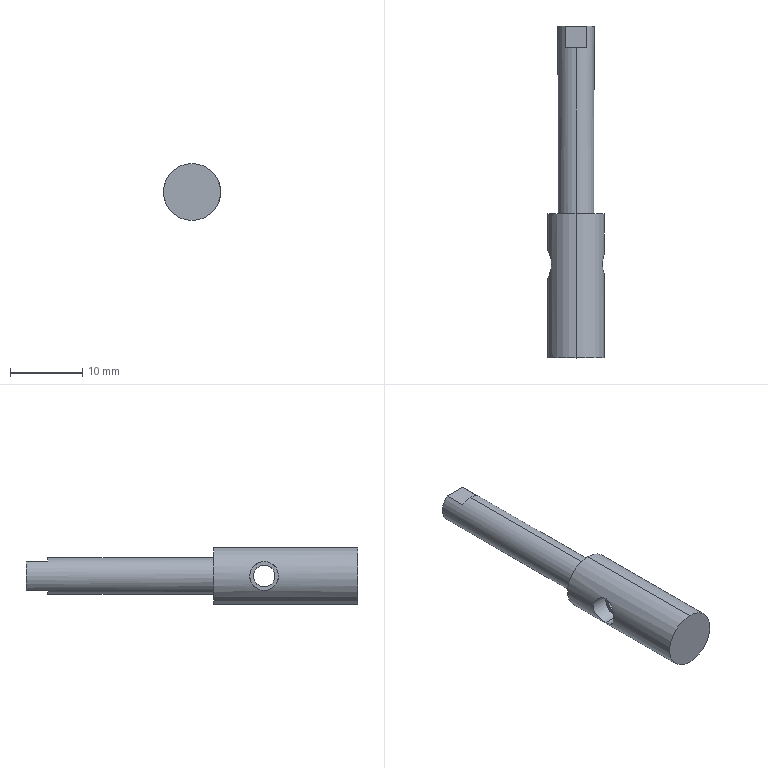Part | SolidWorks | features ICE 4, 3DProfileFeature 1, Extrusion 1, HoleWzd 1 | 1 solid | 20 faces | box 7.9 x 46 x 7.9 mm | volume 1380 mm3 | cylinder 10 | plane 8 | cone 2 | commonest cylinder face diameters 2.5 x2 3 x2 4 x2 5 x2 7.9 x2
STEP:
#1=CARTESIAN_POINT('',(0.,38.5,-1.25));
#2=VERTEX_POINT('',#1);
#3=CARTESIAN_POINT('',(0.,38.5,1.25));
#4=VERTEX_POINT('',#3);
#5=CARTESIAN_POINT('',(0.,38.5,0.));
#6=DIRECTION('',(0.,1.,0.));
#7=DIRECTION('',(0.,0.,1.));
#8=AXIS2_PLACEMENT_3D('',#5,#6,#7);
#9=CIRCLE('',#8,1.25);
#10=EDGE_CURVE('',#2,#4,#9,.T.);
#11=ORIENTED_EDGE('',*,*,#10,.F.);
#12=CARTESIAN_POINT('',(0.,46.,-1.25));
#13=VERTEX_POINT('',#12);
#14=CARTESIAN_POINT('',(0.,46.,-1.25));
#15=DIRECTION('',(0.,1.,0.));
#16=VECTOR('',#15,1000.);
#17=LINE('',#14,#16);
#18=EDGE_CURVE('',#2,#13,#17,.T.);
#19=ORIENTED_EDGE('',*,*,#18,.T.);
#20=CARTESIAN_POINT('',(0.,46.,1.25));
#21=VERTEX_POINT('',#20);
#22=CARTESIAN_POINT('',(0.,46.,0.));
#23=DIRECTION('',(0.,1.,0.));
#24=DIRECTION('',(0.,0.,1.));
#25=AXIS2_PLACEMENT_3D('',#22,#23,#24);
#26=CIRCLE('',#25,1.25);
#27=EDGE_CURVE('',#13,#21,#26,.T.);
#28=ORIENTED_EDGE('',*,*,#27,.T.);
#29=CARTESIAN_POINT('',(0.,46.,1.25));
#30=DIRECTION('',(0.,1.,0.));
#31=VECTOR('',#30,1000.);
#32=LINE('',#29,#31);
#33=EDGE_CURVE('',#4,#21,#32,.T.);
#34=ORIENTED_EDGE('',*,*,#33,.F.);
#35=EDGE_LOOP('',(#11,#19,#28,#34));
#36=FACE_OUTER_BOUND('',#35,.T.);
#37=CARTESIAN_POINT('',(0.,46.,0.));
#38=DIRECTION('',(0.,1.,0.));
#39=DIRECTION('',(0.,0.,1.));
#40=AXIS2_PLACEMENT_3D('',#37,#38,#39);
#41=CYLINDRICAL_SURFACE('',#40,1.25);
#42=ADVANCED_FACE('',(#36),#41,.F.);
#43=CARTESIAN_POINT('',(0.,37.749,0.));
#44=VERTEX_POINT('',#43);
#45=CARTESIAN_POINT('',(0.,38.5,1.25));
#46=DIRECTION('',(0.,0.515,0.8572));
#47=VECTOR('',#46,1000.);
#48=LINE('',#45,#47);
#49=EDGE_CURVE('',#44,#4,#48,.T.);
#50=ORIENTED_EDGE('',*,*,#49,.F.);
#51=CARTESIAN_POINT('',(0.,38.5,-1.25));
#52=DIRECTION('',(0.,0.515,-0.8572));
#53=VECTOR('',#52,1000.);
#54=LINE('',#51,#53);
#55=EDGE_CURVE('',#44,#2,#54,.T.);
#56=ORIENTED_EDGE('',*,*,#55,.T.);
#57=ORIENTED_EDGE('',*,*,#10,.T.);
#58=EDGE_LOOP('',(#50,#56,#57));
#59=FACE_OUTER_BOUND('',#58,.T.);
#60=CARTESIAN_POINT('',(0.,38.5,0.));
#61=DIRECTION('',(0.,1.,0.));
#62=DIRECTION('',(0.,0.,1.));
#63=AXIS2_PLACEMENT_3D('',#60,#61,#62);
#64=CONICAL_SURFACE('',#63,1.25,1.03);
#65=ADVANCED_FACE('',(#59),#64,.F.);
#66=CARTESIAN_POINT('',(-3.406,13.,2.));
#67=VERTEX_POINT('',#66);
#68=CARTESIAN_POINT('',(-3.406,13.,-2.));
#69=VERTEX_POINT('',#68);
#70=CARTESIAN_POINT('',(-3.406,13.,2.));
#71=CARTESIAN_POINT('',(-3.406,12.868,2.));
#72=CARTESIAN_POINT('',(-3.414,12.733,1.986));
#73=CARTESIAN_POINT('',(-3.444,12.473,1.934));
#74=CARTESIAN_POINT('',(-3.466,12.348,1.895));
#75=CARTESIAN_POINT('',(-3.52,12.105,1.793));
#76=CARTESIAN_POINT('',(-3.551,11.991,1.732));
#77=CARTESIAN_POINT('',(-3.618,11.777,1.588));
#78=CARTESIAN_POINT('',(-3.653,11.677,1.505));
#79=CARTESIAN_POINT('',(-3.723,11.495,1.324));
#80=CARTESIAN_POINT('',(-3.757,11.414,1.225));
#81=CARTESIAN_POINT('',(-3.82,11.269,1.01));
#82=CARTESIAN_POINT('',(-3.849,11.206,0.8939));
#83=CARTESIAN_POINT('',(-3.921,11.055,0.5341));
#84=CARTESIAN_POINT('',(-3.95,11.,0.2668));
#85=CARTESIAN_POINT('',(-3.95,11.,-0.1306));
#86=CARTESIAN_POINT('',(-3.943,11.013,-0.2652));
#87=CARTESIAN_POINT('',(-3.917,11.066,-0.5255));
#88=CARTESIAN_POINT('',(-3.898,11.104,-0.6512));
#89=CARTESIAN_POINT('',(-3.825,11.257,-1.015));
#90=CARTESIAN_POINT('',(-3.758,11.404,-1.233));
#91=CARTESIAN_POINT('',(-3.653,11.678,-1.506));
#92=CARTESIAN_POINT('',(-3.618,11.777,-1.588));
#93=CARTESIAN_POINT('',(-3.551,11.991,-1.731));
#94=CARTESIAN_POINT('',(-3.519,12.107,-1.794));
#95=CARTESIAN_POINT('',(-3.466,12.347,-1.895));
#96=CARTESIAN_POINT('',(-3.445,12.471,-1.933));
#97=CARTESIAN_POINT('',(-3.414,12.73,-1.986));
#98=CARTESIAN_POINT('',(-3.406,12.866,-2.));
#99=CARTESIAN_POINT('',(-3.406,13.,-2.));
#100=B_SPLINE_CURVE_WITH_KNOTS('',3,(#70,#71,#72,#73,#74,#75,#76,#77,#78,#79,#80,#81,#82,#83,#84,#85,#86,#87,#88,#89,#90,#91,#92,#93,#94,#95,#96,#97,#98,#99),.UNSPECIFIED.,.F.,.F.,(4,2,2,2,2,2,2,2,2,2,2,2,2,2,4),(0.006364,0.006761,0.007158,0.007555,0.007952,0.008349,0.008746,0.009541,0.009938,0.01033,0.01113,0.01153,0.01192,0.01232,0.01272),.UNSPECIFIED.);
#101=EDGE_CURVE('',#67,#69,#100,.T.);
#102=ORIENTED_EDGE('',*,*,#101,.F.);
#103=CARTESIAN_POINT('',(-1.5,13.,2.));
#104=VERTEX_POINT('',#103);
#105=CARTESIAN_POINT('',(-11.5,13.,2.));
#106=DIRECTION('',(1.,0.,0.));
#107=VECTOR('',#106,1000.);
#108=LINE('',#105,#107);
#109=EDGE_CURVE('',#67,#104,#108,.T.);
#110=ORIENTED_EDGE('',*,*,#109,.T.);
#111=CARTESIAN_POINT('',(-1.5,13.,-2.));
#112=VERTEX_POINT('',#111);
#113=CARTESIAN_POINT('',(-1.5,13.,0.));
#114=DIRECTION('',(1.,0.,0.));
#115=DIRECTION('',(0.,0.,-1.));
#116=AXIS2_PLACEMENT_3D('',#113,#114,#115);
#117=CIRCLE('',#116,2.);
#118=EDGE_CURVE('',#104,#112,#117,.T.);
#119=ORIENTED_EDGE('',*,*,#118,.T.);
#120=CARTESIAN_POINT('',(-11.5,13.,-2.));
#121=DIRECTION('',(1.,0.,0.));
#122=VECTOR('',#121,1000.);
#123=LINE('',#120,#122);
#124=EDGE_CURVE('',#69,#112,#123,.T.);
#125=ORIENTED_EDGE('',*,*,#124,.F.);
#126=EDGE_LOOP('',(#102,#110,#119,#125));
#127=FACE_OUTER_BOUND('',#126,.T.);
#128=CARTESIAN_POINT('',(-11.5,13.,0.));
#129=DIRECTION('',(1.,0.,0.));
#130=DIRECTION('',(0.,0.,-1.));
#131=AXIS2_PLACEMENT_3D('',#128,#129,#130);
#132=CYLINDRICAL_SURFACE('',#131,2.);
#133=ADVANCED_FACE('',(#127),#132,.F.);
#134=CARTESIAN_POINT('',(-1.5,13.,-1.5));
#135=VERTEX_POINT('',#134);
#136=CARTESIAN_POINT('',(-1.5,13.,1.5));
#137=VERTEX_POINT('',#136);
#138=CARTESIAN_POINT('',(-1.5,13.,0.));
#139=DIRECTION('',(-1.,0.,0.));
#140=DIRECTION('',(0.,0.,-1.));
#141=AXIS2_PLACEMENT_3D('',#138,#139,#140);
#142=CIRCLE('',#141,1.5);
#143=EDGE_CURVE('',#135,#137,#142,.T.);
#144=ORIENTED_EDGE('',*,*,#143,.T.);
#145=CARTESIAN_POINT('',(3.654,13.,1.5));
#146=VERTEX_POINT('',#145);
#147=CARTESIAN_POINT('',(-3.95,13.,1.5));
#148=DIRECTION('',(1.,0.,0.));
#149=VECTOR('',#148,1000.);
#150=LINE('',#147,#149);
#151=EDGE_CURVE('',#137,#146,#150,.T.);
#152=ORIENTED_EDGE('',*,*,#151,.T.);
#153=CARTESIAN_POINT('',(3.654,13.,-1.5));
#154=VERTEX_POINT('',#153);
#155=CARTESIAN_POINT('',(3.654,13.,-1.5));
#156=CARTESIAN_POINT('',(3.654,12.9,-1.5));
#157=CARTESIAN_POINT('',(3.658,12.802,-1.49));
#158=CARTESIAN_POINT('',(3.674,12.609,-1.451));
#159=CARTESIAN_POINT('',(3.685,12.513,-1.422));
#160=CARTESIAN_POINT('',(3.728,12.241,-1.309));
#161=CARTESIAN_POINT('',(3.767,12.076,-1.198));
#162=CARTESIAN_POINT('',(3.843,11.802,-0.9235));
#163=CARTESIAN_POINT('',(3.881,11.691,-0.7578));
#164=CARTESIAN_POINT('',(3.921,11.578,-0.4874));
#165=CARTESIAN_POINT('',(3.932,11.549,-0.3918));
#166=CARTESIAN_POINT('',(3.946,11.51,-0.1977));
#167=CARTESIAN_POINT('',(3.95,11.5,-0.09969));
#168=CARTESIAN_POINT('',(3.95,11.5,0.0982));
#169=CARTESIAN_POINT('',(3.946,11.51,0.1986));
#170=CARTESIAN_POINT('',(3.932,11.549,0.3919));
#171=CARTESIAN_POINT('',(3.921,11.577,0.486));
#172=CARTESIAN_POINT('',(3.894,11.654,0.6689));
#173=CARTESIAN_POINT('',(3.878,11.7,0.755));
#174=CARTESIAN_POINT('',(3.843,11.809,0.9166));
#175=CARTESIAN_POINT('',(3.824,11.871,0.9929));
#176=CARTESIAN_POINT('',(3.785,12.009,1.13));
#177=CARTESIAN_POINT('',(3.766,12.084,1.192));
#178=CARTESIAN_POINT('',(3.73,12.246,1.3));
#179=CARTESIAN_POINT('',(3.713,12.333,1.347));
#180=CARTESIAN_POINT('',(3.671,12.604,1.46));
#181=CARTESIAN_POINT('',(3.654,12.803,1.5));
#182=CARTESIAN_POINT('',(3.654,13.,1.5));
#183=B_SPLINE_CURVE_WITH_KNOTS('',3,(#155,#156,#157,#158,#159,#160,#161,#162,#163,#164,#165,#166,#167,#168,#169,#170,#171,#172,#173,#174,#175,#176,#177,#178,#179,#180,#181,#182),.UNSPECIFIED.,.F.,.F.,(4,2,2,2,2,2,2,2,2,2,2,2,2,4),(0.,0.0002959,0.0005918,0.001184,0.001775,0.002071,0.002367,0.002663,0.002959,0.003255,0.003551,0.003847,0.004143,0.004734),.UNSPECIFIED.);
#184=EDGE_CURVE('',#154,#146,#183,.T.);
#185=ORIENTED_EDGE('',*,*,#184,.F.);
#186=CARTESIAN_POINT('',(-3.95,13.,-1.5));
#187=DIRECTION('',(1.,0.,0.));
#188=VECTOR('',#187,1000.);
#189=LINE('',#186,#188);
#190=EDGE_CURVE('',#135,#154,#189,.T.);
#191=ORIENTED_EDGE('',*,*,#190,.F.);
#192=EDGE_LOOP('',(#144,#152,#185,#191));
#193=FACE_OUTER_BOUND('',#192,.T.);
#194=CARTESIAN_POINT('',(-3.95,13.,0.));
#195=DIRECTION('',(1.,0.,0.));
#196=DIRECTION('',(0.,0.,-1.));
#197=AXIS2_PLACEMENT_3D('',#194,#195,#196);
#198=CYLINDRICAL_SURFACE('',#197,1.5);
#199=ADVANCED_FACE('',(#193),#198,.F.);
#200=ORIENTED_EDGE('',*,*,#184,.T.);
#201=CARTESIAN_POINT('',(3.654,13.,1.5));
#202=CARTESIAN_POINT('',(3.654,13.197,1.5));
#203=CARTESIAN_POINT('',(3.671,13.396,1.46));
#204=CARTESIAN_POINT('',(3.714,13.668,1.347));
#205=CARTESIAN_POINT('',(3.73,13.755,1.3));
#206=CARTESIAN_POINT('',(3.766,13.917,1.191));
#207=CARTESIAN_POINT('',(3.786,13.992,1.13));
#208=CARTESIAN_POINT('',(3.824,14.13,0.9909));
#209=CARTESIAN_POINT('',(3.843,14.192,0.9158));
#210=CARTESIAN_POINT('',(3.878,14.3,0.7545));
#211=CARTESIAN_POINT('',(3.894,14.347,0.6672));
#212=CARTESIAN_POINT('',(3.921,14.423,0.4855));
#213=CARTESIAN_POINT('',(3.932,14.451,0.3918));
#214=CARTESIAN_POINT('',(3.946,14.49,0.1986));
#215=CARTESIAN_POINT('',(3.95,14.5,0.09808));
#216=CARTESIAN_POINT('',(3.95,14.5,-0.1985));
#217=CARTESIAN_POINT('',(3.934,14.46,-0.3974));
#218=CARTESIAN_POINT('',(3.881,14.309,-0.7587));
#219=CARTESIAN_POINT('',(3.843,14.197,-0.9241));
#220=CARTESIAN_POINT('',(3.786,13.991,-1.13));
#221=CARTESIAN_POINT('',(3.766,13.915,-1.193));
#222=CARTESIAN_POINT('',(3.73,13.753,-1.301));
#223=CARTESIAN_POINT('',(3.713,13.667,-1.347));
#224=CARTESIAN_POINT('',(3.671,13.394,-1.461));
#225=CARTESIAN_POINT('',(3.654,13.2,-1.5));
#226=CARTESIAN_POINT('',(3.654,13.,-1.5));
#227=B_SPLINE_CURVE_WITH_KNOTS('',3,(#201,#202,#203,#204,#205,#206,#207,#208,#209,#210,#211,#212,#213,#214,#215,#216,#217,#218,#219,#220,#221,#222,#223,#224,#225,#226),.UNSPECIFIED.,.F.,.F.,(4,2,2,2,2,2,2,2,2,2,2,2,4),(0.004734,0.005326,0.005622,0.005918,0.006214,0.006509,0.006805,0.007101,0.007693,0.008284,0.00858,0.008876,0.009468),.UNSPECIFIED.);
#228=EDGE_CURVE('',#146,#154,#227,.T.);
#229=ORIENTED_EDGE('',*,*,#228,.T.);
#230=EDGE_LOOP('',(#200,#229));
#231=FACE_BOUND('',#230,.T.);
#232=CARTESIAN_POINT('',(0.,20.,3.95));
#233=VERTEX_POINT('',#232);
#234=CARTESIAN_POINT('',(0.,20.,-3.95));
#235=VERTEX_POINT('',#234);
#236=CARTESIAN_POINT('',(0.,20.,0.));
#237=DIRECTION('',(0.,1.,0.));
#238=DIRECTION('',(0.,0.,1.));
#239=AXIS2_PLACEMENT_3D('',#236,#237,#238);
#240=CIRCLE('',#239,3.95);
#241=EDGE_CURVE('',#233,#235,#240,.T.);
#242=ORIENTED_EDGE('',*,*,#241,.F.);
#243=CARTESIAN_POINT('',(0.,0.,3.95));
#244=VERTEX_POINT('',#243);
#245=CARTESIAN_POINT('',(0.,20.,3.95));
#246=DIRECTION('',(0.,-1.,0.));
#247=VECTOR('',#246,1000.);
#248=LINE('',#245,#247);
#249=EDGE_CURVE('',#233,#244,#248,.T.);
#250=ORIENTED_EDGE('',*,*,#249,.T.);
#251=CARTESIAN_POINT('',(0.,0.,-3.95));
#252=VERTEX_POINT('',#251);
#253=CARTESIAN_POINT('',(0.,0.,0.));
#254=DIRECTION('',(0.,1.,0.));
#255=DIRECTION('',(0.,0.,1.));
#256=AXIS2_PLACEMENT_3D('',#253,#254,#255);
#257=CIRCLE('',#256,3.95);
#258=EDGE_CURVE('',#244,#252,#257,.T.);
#259=ORIENTED_EDGE('',*,*,#258,.T.);
#260=CARTESIAN_POINT('',(0.,20.,-3.95));
#261=DIRECTION('',(0.,-1.,0.));
#262=VECTOR('',#261,1000.);
#263=LINE('',#260,#262);
#264=EDGE_CURVE('',#235,#252,#263,.T.);
#265=ORIENTED_EDGE('',*,*,#264,.F.);
#266=EDGE_LOOP('',(#242,#250,#259,#265));
#267=FACE_OUTER_BOUND('',#266,.T.);
#268=CARTESIAN_POINT('',(0.,20.,0.));
#269=DIRECTION('',(0.,-1.,0.));
#270=DIRECTION('',(0.,0.,-1.));
#271=AXIS2_PLACEMENT_3D('',#268,#269,#270);
#272=CYLINDRICAL_SURFACE('',#271,3.95);
#273=ADVANCED_FACE('',(#231,#267),#272,.T.);
#274=CARTESIAN_POINT('',(0.,43.,2.5));
#275=VERTEX_POINT('',#274);
#276=CARTESIAN_POINT('',(1.5,43.,2.));
#277=VERTEX_POINT('',#276);
#278=CARTESIAN_POINT('',(0.,43.,0.));
#279=DIRECTION('',(0.,1.,0.));
#280=DIRECTION('',(0.,0.,1.));
#281=AXIS2_PLACEMENT_3D('',#278,#279,#280);
#282=CIRCLE('',#281,2.5);
#283=EDGE_CURVE('',#275,#277,#282,.T.);
#284=ORIENTED_EDGE('',*,*,#283,.F.);
#285=CARTESIAN_POINT('',(0.,20.,2.5));
#286=VERTEX_POINT('',#285);
#287=CARTESIAN_POINT('',(0.,46.,2.5));
#288=DIRECTION('',(0.,-1.,0.));
#289=VECTOR('',#288,1000.);
#290=LINE('',#287,#289);
#291=EDGE_CURVE('',#275,#286,#290,.T.);
#292=ORIENTED_EDGE('',*,*,#291,.T.);
#293=CARTESIAN_POINT('',(0.,20.,-2.5));
#294=VERTEX_POINT('',#293);
#295=CARTESIAN_POINT('',(0.,20.,0.));
#296=DIRECTION('',(0.,1.,0.));
#297=DIRECTION('',(0.,0.,1.));
#298=AXIS2_PLACEMENT_3D('',#295,#296,#297);
#299=CIRCLE('',#298,2.5);
#300=EDGE_CURVE('',#286,#294,#299,.T.);
#301=ORIENTED_EDGE('',*,*,#300,.T.);
#302=CARTESIAN_POINT('',(0.,43.,-2.5));
#303=VERTEX_POINT('',#302);
#304=CARTESIAN_POINT('',(0.,46.,-2.5));
#305=DIRECTION('',(0.,-1.,0.));
#306=VECTOR('',#305,1000.);
#307=LINE('',#304,#306);
#308=EDGE_CURVE('',#303,#294,#307,.T.);
#309=ORIENTED_EDGE('',*,*,#308,.F.);
#310=CARTESIAN_POINT('',(1.5,43.,-2.));
#311=VERTEX_POINT('',#310);
#312=CARTESIAN_POINT('',(0.,43.,0.));
#313=DIRECTION('',(0.,1.,0.));
#314=DIRECTION('',(0.,0.,1.));
#315=AXIS2_PLACEMENT_3D('',#312,#313,#314);
#316=CIRCLE('',#315,2.5);
#317=EDGE_CURVE('',#311,#303,#316,.T.);
#318=ORIENTED_EDGE('',*,*,#317,.F.);
#319=CARTESIAN_POINT('',(1.5,46.,-2.));
#320=VERTEX_POINT('',#319);
#321=CARTESIAN_POINT('',(1.5,46.,-2.));
#322=DIRECTION('',(0.,-1.,0.));
#323=VECTOR('',#322,1000.);
#324=LINE('',#321,#323);
#325=EDGE_CURVE('',#320,#311,#324,.T.);
#326=ORIENTED_EDGE('',*,*,#325,.F.);
#327=CARTESIAN_POINT('',(1.5,46.,2.));
#328=VERTEX_POINT('',#327);
#329=CARTESIAN_POINT('',(0.,46.,0.));
#330=DIRECTION('',(0.,1.,0.));
#331=DIRECTION('',(0.,0.,1.));
#332=AXIS2_PLACEMENT_3D('',#329,#330,#331);
#333=CIRCLE('',#332,2.5);
#334=EDGE_CURVE('',#328,#320,#333,.T.);
#335=ORIENTED_EDGE('',*,*,#334,.F.);
#336=CARTESIAN_POINT('',(1.5,46.,2.));
#337=DIRECTION('',(0.,1.,0.));
#338=VECTOR('',#337,1000.);
#339=LINE('',#336,#338);
#340=EDGE_CURVE('',#277,#328,#339,.T.);
#341=ORIENTED_EDGE('',*,*,#340,.F.);
#342=EDGE_LOOP('',(#284,#292,#301,#309,#318,#326,#335,#341));
#343=FACE_OUTER_BOUND('',#342,.T.);
#344=CARTESIAN_POINT('',(0.,46.,0.));
#345=DIRECTION('',(0.,-1.,0.));
#346=DIRECTION('',(0.,0.,-1.));
#347=AXIS2_PLACEMENT_3D('',#344,#345,#346);
#348=CYLINDRICAL_SURFACE('',#347,2.5);
#349=ADVANCED_FACE('',(#343),#348,.T.);
#350=ORIENTED_EDGE('',*,*,#291,.F.);
#351=CARTESIAN_POINT('',(-1.5,43.,2.));
#352=VERTEX_POINT('',#351);
#353=CARTESIAN_POINT('',(0.,43.,0.));
#354=DIRECTION('',(0.,1.,0.));
#355=DIRECTION('',(0.,0.,1.));
#356=AXIS2_PLACEMENT_3D('',#353,#354,#355);
#357=CIRCLE('',#356,2.5);
#358=EDGE_CURVE('',#352,#275,#357,.T.);
#359=ORIENTED_EDGE('',*,*,#358,.F.);
#360=CARTESIAN_POINT('',(-1.5,46.,2.));
#361=VERTEX_POINT('',#360);
#362=CARTESIAN_POINT('',(-1.5,46.,2.));
#363=DIRECTION('',(0.,-1.,0.));
#364=VECTOR('',#363,1000.);
#365=LINE('',#362,#364);
#366=EDGE_CURVE('',#361,#352,#365,.T.);
#367=ORIENTED_EDGE('',*,*,#366,.F.);
#368=CARTESIAN_POINT('',(-1.5,46.,-2.));
#369=VERTEX_POINT('',#368);
#370=CARTESIAN_POINT('',(0.,46.,0.));
#371=DIRECTION('',(0.,1.,0.));
#372=DIRECTION('',(0.,0.,1.));
#373=AXIS2_PLACEMENT_3D('',#370,#371,#372);
#374=CIRCLE('',#373,2.5);
#375=EDGE_CURVE('',#369,#361,#374,.T.);
#376=ORIENTED_EDGE('',*,*,#375,.F.);
#377=CARTESIAN_POINT('',(-1.5,43.,-2.));
#378=VERTEX_POINT('',#377);
#379=CARTESIAN_POINT('',(-1.5,46.,-2.));
#380=DIRECTION('',(0.,1.,0.));
#381=VECTOR('',#380,1000.);
#382=LINE('',#379,#381);
#383=EDGE_CURVE('',#378,#369,#382,.T.);
#384=ORIENTED_EDGE('',*,*,#383,.F.);
#385=CARTESIAN_POINT('',(0.,43.,0.));
#386=DIRECTION('',(0.,1.,0.));
#387=DIRECTION('',(0.,0.,1.));
#388=AXIS2_PLACEMENT_3D('',#385,#386,#387);
#389=CIRCLE('',#388,2.5);
#390=EDGE_CURVE('',#303,#378,#389,.T.);
#391=ORIENTED_EDGE('',*,*,#390,.F.);
#392=ORIENTED_EDGE('',*,*,#308,.T.);
#393=CARTESIAN_POINT('',(0.,20.,0.));
#394=DIRECTION('',(0.,1.,0.));
#395=DIRECTION('',(0.,0.,1.));
#396=AXIS2_PLACEMENT_3D('',#393,#394,#395);
#397=CIRCLE('',#396,2.5);
#398=EDGE_CURVE('',#294,#286,#397,.T.);
#399=ORIENTED_EDGE('',*,*,#398,.T.);
#400=EDGE_LOOP('',(#350,#359,#367,#376,#384,#391,#392,#399));
#401=FACE_OUTER_BOUND('',#400,.T.);
#402=CARTESIAN_POINT('',(0.,46.,0.));
#403=DIRECTION('',(0.,-1.,0.));
#404=DIRECTION('',(0.,0.,-1.));
#405=AXIS2_PLACEMENT_3D('',#402,#403,#404);
#406=CYLINDRICAL_SURFACE('',#405,2.5);
#407=ADVANCED_FACE('',(#401),#406,.T.);
#408=CARTESIAN_POINT('',(0.,46.,0.));
#409=DIRECTION('',(0.,1.,0.));
#410=DIRECTION('',(0.,0.,1.));
#411=AXIS2_PLACEMENT_3D('',#408,#409,#410);
#412=CIRCLE('',#411,1.25);
#413=EDGE_CURVE('',#21,#13,#412,.T.);
#414=ORIENTED_EDGE('',*,*,#413,.F.);
#415=ORIENTED_EDGE('',*,*,#27,.F.);
#416=EDGE_LOOP('',(#414,#415));
#417=FACE_BOUND('',#416,.T.);
#418=ORIENTED_EDGE('',*,*,#375,.T.);
#419=CARTESIAN_POINT('',(0.,46.,2.));
#420=DIRECTION('',(1.,0.,0.));
#421=VECTOR('',#420,1000.);
#422=LINE('',#419,#421);
#423=EDGE_CURVE('',#361,#328,#422,.T.);
#424=ORIENTED_EDGE('',*,*,#423,.T.);
#425=ORIENTED_EDGE('',*,*,#334,.T.);
#426=CARTESIAN_POINT('',(0.,46.,-2.));
#427=DIRECTION('',(-1.,0.,0.));
#428=VECTOR('',#427,1000.);
#429=LINE('',#426,#428);
#430=EDGE_CURVE('',#320,#369,#429,.T.);
#431=ORIENTED_EDGE('',*,*,#430,.T.);
#432=EDGE_LOOP('',(#418,#424,#425,#431));
#433=FACE_OUTER_BOUND('',#432,.T.);
#434=CARTESIAN_POINT('',(0.,46.,0.));
#435=DIRECTION('',(0.,1.,0.));
#436=DIRECTION('',(0.,0.,1.));
#437=AXIS2_PLACEMENT_3D('',#434,#435,#436);
#438=PLANE('',#437);
#439=ADVANCED_FACE('',(#417,#433),#438,.T.);
#440=ORIENTED_EDGE('',*,*,#249,.F.);
#441=CARTESIAN_POINT('',(0.,20.,0.));
#442=DIRECTION('',(0.,1.,0.));
#443=DIRECTION('',(0.,0.,1.));
#444=AXIS2_PLACEMENT_3D('',#441,#442,#443);
#445=CIRCLE('',#444,3.95);
#446=EDGE_CURVE('',#235,#233,#445,.T.);
#447=ORIENTED_EDGE('',*,*,#446,.F.);
#448=ORIENTED_EDGE('',*,*,#264,.T.);
#449=CARTESIAN_POINT('',(0.,0.,0.));
#450=DIRECTION('',(0.,1.,0.));
#451=DIRECTION('',(0.,0.,1.));
#452=AXIS2_PLACEMENT_3D('',#449,#450,#451);
#453=CIRCLE('',#452,3.95);
#454=EDGE_CURVE('',#252,#244,#453,.T.);
#455=ORIENTED_EDGE('',*,*,#454,.T.);
#456=EDGE_LOOP('',(#440,#447,#448,#455));
#457=FACE_OUTER_BOUND('',#456,.T.);
#458=CARTESIAN_POINT('',(-3.406,13.,-2.));
#459=CARTESIAN_POINT('',(-3.406,13.135,-2.));
#460=CARTESIAN_POINT('',(-3.414,13.267,-1.987));
#461=CARTESIAN_POINT('',(-3.444,13.525,-1.934));
#462=CARTESIAN_POINT('',(-3.466,13.653,-1.895));
#463=CARTESIAN_POINT('',(-3.546,14.014,-1.743));
#464=CARTESIAN_POINT('',(-3.618,14.232,-1.596));
#465=CARTESIAN_POINT('',(-3.757,14.595,-1.234));
#466=CARTESIAN_POINT('',(-3.825,14.743,-1.015));
#467=CARTESIAN_POINT('',(-3.897,14.894,-0.6542));
#468=CARTESIAN_POINT('',(-3.917,14.934,-0.5258));
#469=CARTESIAN_POINT('',(-3.943,14.987,-0.2663));
#470=CARTESIAN_POINT('',(-3.95,15.,-0.1347));
#471=CARTESIAN_POINT('',(-3.95,15.,0.132));
#472=CARTESIAN_POINT('',(-3.943,14.987,0.2667));
#473=CARTESIAN_POINT('',(-3.917,14.934,0.5259));
#474=CARTESIAN_POINT('',(-3.898,14.895,0.6533));
#475=CARTESIAN_POINT('',(-3.849,14.793,0.8961));
#476=CARTESIAN_POINT('',(-3.82,14.731,1.01));
#477=CARTESIAN_POINT('',(-3.757,14.586,1.225));
#478=CARTESIAN_POINT('',(-3.722,14.503,1.326));
#479=CARTESIAN_POINT('',(-3.618,14.23,1.598));
#480=CARTESIAN_POINT('',(-3.545,14.011,1.745));
#481=CARTESIAN_POINT('',(-3.466,13.652,1.895));
#482=CARTESIAN_POINT('',(-3.444,13.525,1.934));
#483=CARTESIAN_POINT('',(-3.414,13.264,1.987));
#484=CARTESIAN_POINT('',(-3.406,13.133,2.));
#485=CARTESIAN_POINT('',(-3.406,13.,2.));
#486=B_SPLINE_CURVE_WITH_KNOTS('',3,(#458,#459,#460,#461,#462,#463,#464,#465,#466,#467,#468,#469,#470,#471,#472,#473,#474,#475,#476,#477,#478,#479,#480,#481,#482,#483,#484,#485),.UNSPECIFIED.,.F.,.F.,(4,2,2,2,2,2,2,2,2,2,2,2,2,4),(0.,0.0003978,0.0007955,0.001591,0.002387,0.002784,0.003182,0.00358,0.003978,0.004375,0.004773,0.005569,0.005967,0.006364),.UNSPECIFIED.);
#487=EDGE_CURVE('',#69,#67,#486,.T.);
#488=ORIENTED_EDGE('',*,*,#487,.T.);
#489=ORIENTED_EDGE('',*,*,#101,.T.);
#490=EDGE_LOOP('',(#488,#489));
#491=FACE_BOUND('',#490,.T.);
#492=CARTESIAN_POINT('',(0.,20.,0.));
#493=DIRECTION('',(0.,-1.,0.));
#494=DIRECTION('',(0.,0.,-1.));
#495=AXIS2_PLACEMENT_3D('',#492,#493,#494);
#496=CYLINDRICAL_SURFACE('',#495,3.95);
#497=ADVANCED_FACE('',(#457,#491),#496,.T.);
#498=ORIENTED_EDGE('',*,*,#398,.F.);
#499=ORIENTED_EDGE('',*,*,#300,.F.);
#500=EDGE_LOOP('',(#498,#499));
#501=FACE_BOUND('',#500,.T.);
#502=ORIENTED_EDGE('',*,*,#446,.T.);
#503=ORIENTED_EDGE('',*,*,#241,.T.);
#504=EDGE_LOOP('',(#502,#503));
#505=FACE_OUTER_BOUND('',#504,.T.);
#506=CARTESIAN_POINT('',(0.,20.,0.));
#507=DIRECTION('',(0.,1.,0.));
#508=DIRECTION('',(0.,0.,1.));
#509=AXIS2_PLACEMENT_3D('',#506,#507,#508);
#510=PLANE('',#509);
#511=ADVANCED_FACE('',(#501,#505),#510,.T.);
#512=ORIENTED_EDGE('',*,*,#454,.F.);
#513=ORIENTED_EDGE('',*,*,#258,.F.);
#514=EDGE_LOOP('',(#512,#513));
#515=FACE_OUTER_BOUND('',#514,.T.);
#516=CARTESIAN_POINT('',(0.,0.,0.));
#517=DIRECTION('',(0.,1.,0.));
#518=DIRECTION('',(0.,0.,1.));
#519=AXIS2_PLACEMENT_3D('',#516,#517,#518);
#520=PLANE('',#519);
#521=ADVANCED_FACE('',(#515),#520,.F.);
#522=ORIENTED_EDGE('',*,*,#325,.T.);
#523=CARTESIAN_POINT('',(-2.898,43.,-2.));
#524=DIRECTION('',(-1.,0.,0.));
#525=VECTOR('',#524,1000.);
#526=LINE('',#523,#525);
#527=EDGE_CURVE('',#311,#378,#526,.T.);
#528=ORIENTED_EDGE('',*,*,#527,.T.);
#529=ORIENTED_EDGE('',*,*,#383,.T.);
#530=ORIENTED_EDGE('',*,*,#430,.F.);
#531=EDGE_LOOP('',(#522,#528,#529,#530));
#532=FACE_OUTER_BOUND('',#531,.T.);
#533=CARTESIAN_POINT('',(-2.898,43.,-2.));
#534=DIRECTION('',(0.,0.,-1.));
#535=DIRECTION('',(-1.,0.,0.));
#536=AXIS2_PLACEMENT_3D('',#533,#534,#535);
#537=PLANE('',#536);
#538=ADVANCED_FACE('',(#532),#537,.T.);
#539=ORIENTED_EDGE('',*,*,#317,.T.);
#540=ORIENTED_EDGE('',*,*,#390,.T.);
#541=ORIENTED_EDGE('',*,*,#527,.F.);
#542=EDGE_LOOP('',(#539,#540,#541));
#543=FACE_OUTER_BOUND('',#542,.T.);
#544=CARTESIAN_POINT('',(0.,43.,0.));
#545=DIRECTION('',(0.,1.,0.));
#546=DIRECTION('',(0.,0.,1.));
#547=AXIS2_PLACEMENT_3D('',#544,#545,#546);
#548=PLANE('',#547);
#549=ADVANCED_FACE('',(#543),#548,.T.);
#550=ORIENTED_EDGE('',*,*,#358,.T.);
#551=ORIENTED_EDGE('',*,*,#283,.T.);
#552=CARTESIAN_POINT('',(-2.898,43.,2.));
#553=DIRECTION('',(1.,0.,0.));
#554=VECTOR('',#553,1000.);
#555=LINE('',#552,#554);
#556=EDGE_CURVE('',#352,#277,#555,.T.);
#557=ORIENTED_EDGE('',*,*,#556,.F.);
#558=EDGE_LOOP('',(#550,#551,#557));
#559=FACE_OUTER_BOUND('',#558,.T.);
#560=CARTESIAN_POINT('',(0.,43.,0.));
#561=DIRECTION('',(0.,1.,0.));
#562=DIRECTION('',(0.,0.,1.));
#563=AXIS2_PLACEMENT_3D('',#560,#561,#562);
#564=PLANE('',#563);
#565=ADVANCED_FACE('',(#559),#564,.T.);
#566=ORIENTED_EDGE('',*,*,#366,.T.);
#567=ORIENTED_EDGE('',*,*,#556,.T.);
#568=ORIENTED_EDGE('',*,*,#340,.T.);
#569=ORIENTED_EDGE('',*,*,#423,.F.);
#570=EDGE_LOOP('',(#566,#567,#568,#569));
#571=FACE_OUTER_BOUND('',#570,.T.);
#572=CARTESIAN_POINT('',(-2.898,43.,2.));
#573=DIRECTION('',(0.,0.,1.));
#574=DIRECTION('',(1.,0.,0.));
#575=AXIS2_PLACEMENT_3D('',#572,#573,#574);
#576=PLANE('',#575);
#577=ADVANCED_FACE('',(#571),#576,.T.);
#578=ORIENTED_EDGE('',*,*,#151,.F.);
#579=CARTESIAN_POINT('',(-1.5,13.,0.));
#580=DIRECTION('',(-1.,0.,0.));
#581=DIRECTION('',(0.,0.,-1.));
#582=AXIS2_PLACEMENT_3D('',#579,#580,#581);
#583=CIRCLE('',#582,1.5);
#584=EDGE_CURVE('',#137,#135,#583,.T.);
#585=ORIENTED_EDGE('',*,*,#584,.T.);
#586=ORIENTED_EDGE('',*,*,#190,.T.);
#587=ORIENTED_EDGE('',*,*,#228,.F.);
#588=EDGE_LOOP('',(#578,#585,#586,#587));
#589=FACE_OUTER_BOUND('',#588,.T.);
#590=CARTESIAN_POINT('',(-3.95,13.,0.));
#591=DIRECTION('',(1.,0.,0.));
#592=DIRECTION('',(0.,0.,-1.));
#593=AXIS2_PLACEMENT_3D('',#590,#591,#592);
#594=CYLINDRICAL_SURFACE('',#593,1.5);
#595=ADVANCED_FACE('',(#589),#594,.F.);
#596=ORIENTED_EDGE('',*,*,#109,.F.);
#597=ORIENTED_EDGE('',*,*,#487,.F.);
#598=ORIENTED_EDGE('',*,*,#124,.T.);
#599=CARTESIAN_POINT('',(-1.5,13.,0.));
#600=DIRECTION('',(1.,0.,0.));
#601=DIRECTION('',(0.,0.,-1.));
#602=AXIS2_PLACEMENT_3D('',#599,#600,#601);
#603=CIRCLE('',#602,2.);
#604=EDGE_CURVE('',#112,#104,#603,.T.);
#605=ORIENTED_EDGE('',*,*,#604,.T.);
#606=EDGE_LOOP('',(#596,#597,#598,#605));
#607=FACE_OUTER_BOUND('',#606,.T.);
#608=CARTESIAN_POINT('',(-11.5,13.,0.));
#609=DIRECTION('',(1.,0.,0.));
#610=DIRECTION('',(0.,0.,-1.));
#611=AXIS2_PLACEMENT_3D('',#608,#609,#610);
#612=CYLINDRICAL_SURFACE('',#611,2.);
#613=ADVANCED_FACE('',(#607),#612,.F.);
#614=ORIENTED_EDGE('',*,*,#604,.F.);
#615=ORIENTED_EDGE('',*,*,#118,.F.);
#616=EDGE_LOOP('',(#614,#615));
#617=FACE_OUTER_BOUND('',#616,.T.);
#618=ORIENTED_EDGE('',*,*,#143,.F.);
#619=ORIENTED_EDGE('',*,*,#584,.F.);
#620=EDGE_LOOP('',(#618,#619));
#621=FACE_BOUND('',#620,.T.);
#622=CARTESIAN_POINT('',(-1.5,13.,0.));
#623=DIRECTION('',(1.,0.,0.));
#624=DIRECTION('',(0.,0.,-1.));
#625=AXIS2_PLACEMENT_3D('',#622,#623,#624);
#626=PLANE('',#625);
#627=ADVANCED_FACE('',(#617,#621),#626,.F.);
#628=ORIENTED_EDGE('',*,*,#55,.F.);
#629=ORIENTED_EDGE('',*,*,#49,.T.);
#630=CARTESIAN_POINT('',(0.,38.5,0.));
#631=DIRECTION('',(0.,1.,0.));
#632=DIRECTION('',(0.,0.,1.));
#633=AXIS2_PLACEMENT_3D('',#630,#631,#632);
#634=CIRCLE('',#633,1.25);
#635=EDGE_CURVE('',#4,#2,#634,.T.);
#636=ORIENTED_EDGE('',*,*,#635,.T.);
#637=EDGE_LOOP('',(#628,#629,#636));
#638=FACE_OUTER_BOUND('',#637,.T.);
#639=CARTESIAN_POINT('',(0.,38.5,0.));
#640=DIRECTION('',(0.,1.,0.));
#641=DIRECTION('',(0.,0.,1.));
#642=AXIS2_PLACEMENT_3D('',#639,#640,#641);
#643=CONICAL_SURFACE('',#642,1.25,1.03);
#644=ADVANCED_FACE('',(#638),#643,.F.);
#645=ORIENTED_EDGE('',*,*,#18,.F.);
#646=ORIENTED_EDGE('',*,*,#635,.F.);
#647=ORIENTED_EDGE('',*,*,#33,.T.);
#648=ORIENTED_EDGE('',*,*,#413,.T.);
#649=EDGE_LOOP('',(#645,#646,#647,#648));
#650=FACE_OUTER_BOUND('',#649,.T.);
#651=CARTESIAN_POINT('',(0.,46.,0.));
#652=DIRECTION('',(0.,1.,0.));
#653=DIRECTION('',(0.,0.,1.));
#654=AXIS2_PLACEMENT_3D('',#651,#652,#653);
#655=CYLINDRICAL_SURFACE('',#654,1.25);
#656=ADVANCED_FACE('',(#650),#655,.F.);
#657=CLOSED_SHELL('',(#42,#65,#133,#199,#273,#349,#407,#439,#497,#511,#521,#538,#549,#565,#577,#595,#613,#627,#644,#656));
#658=MANIFOLD_SOLID_BREP('',#657);
#659=CARTESIAN_POINT('',(0.,0.,0.));
#660=DIRECTION('',(0.,0.,1.));
#661=DIRECTION('',(1.,0.,0.));
#662=AXIS2_PLACEMENT_3D('',#659,#660,#661);
#663=(LENGTH_UNIT()NAMED_UNIT(*)SI_UNIT(.MILLI.,.METRE.));
#664=UNCERTAINTY_MEASURE_WITH_UNIT(LENGTH_MEASURE(0.00001),#663,'','');
#665=(NAMED_UNIT(*)PLANE_ANGLE_UNIT()SI_UNIT($,.RADIAN.));
#666=(NAMED_UNIT(*)SI_UNIT($,.STERADIAN.)SOLID_ANGLE_UNIT());
#667=(GEOMETRIC_REPRESENTATION_CONTEXT(3)GLOBAL_UNCERTAINTY_ASSIGNED_CONTEXT((#664))GLOBAL_UNIT_ASSIGNED_CONTEXT((#663,#665,#666))REPRESENTATION_CONTEXT('',''));
#668=ADVANCED_BREP_SHAPE_REPRESENTATION('',(#658,#662),#667);